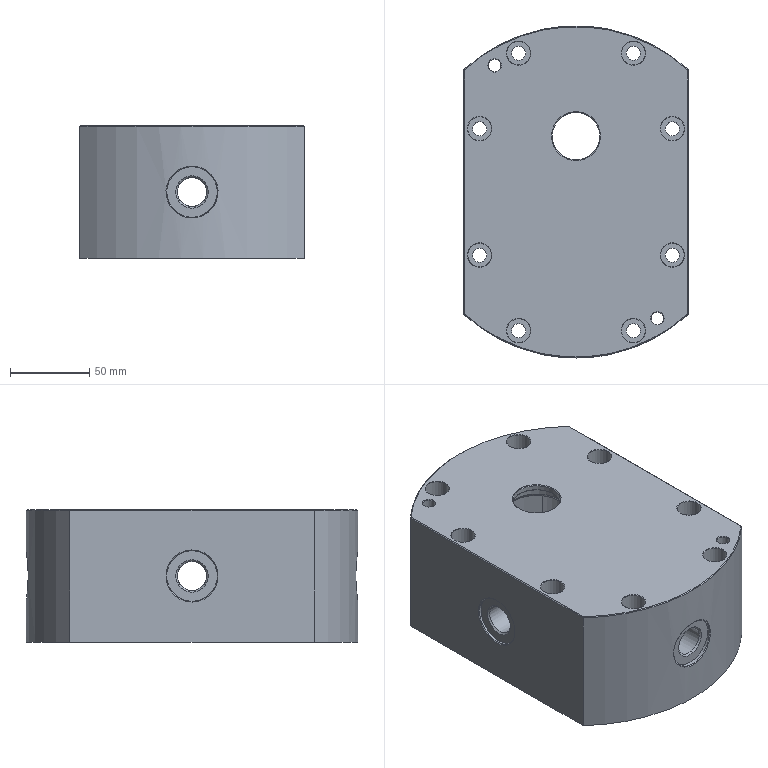NC program | NX | posted with a generic post | part box 142 x 210 x 84 mm
Lines 1512 to 1634 of 1634:
(HOLE_MILLING_COPY_1_COPY_1 , TOOL : D10JING)
N3016 T11 M6
N3018 G54
N3020 G17 G0 G90 X35.25 Y0. B0. C0. S5000 M3
N3022 G43 Z30. H11
N3024 Z-12.
N3026 G94 G1 X32.801 Y-6.451 F1000.
N3028 G3 X35.25 Y-10. R2.619
N3030 X45.25 Y0. R10.
N3032 X35.25 Y-10. R-10.
N3034 X37.699 Y-6.451 R2.619
N3036 G1 X35.25 Y0.
N3038 G0 Z30.
N3040 M5
(PLANAR_MILL_COPY_COPY , TOOL : D6A45)
N3042 T07 M6
N3044 G54
N3046 G17 G0 G90 X92.513 Y-38.084 B0. C0. S7500 M3
N3048 G43 Z30. H7
N3050 Z1.5
N3052 G94 G1 Z-1.5 F1250.
N3054 X93.661 Y-37.121
N3056 G3 X94.019 Y-36.355 R1.
N3058 X87.769 Y-30.105 R6.25
N3060 X94.019 Y-36.355 R-6.25
N3062 X93.661 Y-35.589 R1.
N3064 G1 X92.513 Y-34.625
N3066 Z1.5
N3068 G0 Z30.
N3070 X38.271 Y-65.745
N3072 Z1.5
N3074 G1 Z-1.5
N3076 X39.234 Y-66.893
N3078 G3 X40. Y-67.25 R1.
N3080 X46.25 Y-61. R6.25
N3082 X40. Y-67.25 R-6.25
N3084 X40.766 Y-66.893 R1.
N3086 G1 X41.729 Y-65.745
N3088 Z1.5
N3090 G0 Z30.
N3092 X33.697 Y-12.705
N3094 Z1.5
N3096 G1 Z-1.5
N3098 X34.484 Y-13.643
N3100 G3 X35.25 Y-14. R1.
N3102 X49.25 Y0. R14.
N3104 X35.25 Y-14. R-14.
N3106 X36.016 Y-13.643 R1.
N3108 G1 X36.803 Y-12.705
N3110 Z1.5
N3112 G0 Z30.
N3114 X92.513 Y34.625
N3116 Z1.5
N3118 G1 Z-1.5
N3120 X93.661 Y35.589
N3122 G3 X94.019 Y36.355 R1.
N3124 X87.769 Y42.605 R6.25
N3126 X94.019 Y36.355 R-6.25
N3128 X93.661 Y37.121 R1.
N3130 G1 X92.513 Y38.084
N3132 Z1.5
N3134 G0 Z30.
N3136 X41.729 Y65.745
N3138 Z1.5
N3140 G1 Z-1.5
N3142 X40.766 Y66.893
N3144 G3 X40. Y67.25 R1.
N3146 X33.75 Y61. R6.25
N3148 X40. Y67.25 R-6.25
N3150 X39.234 Y66.893 R1.
N3152 G1 X38.271 Y65.745
N3154 Z1.5
N3156 G0 Z30.
N3158 X-38.271
N3160 Z1.5
N3162 G1 Z-1.5
N3164 X-39.234 Y66.893
N3166 G3 X-40. Y67.25 R1.
N3168 X-46.25 Y61. R6.25
N3170 X-40. Y67.25 R-6.25
N3172 X-40.766 Y66.893 R1.
N3174 G1 X-41.729 Y65.745
N3176 Z1.5
N3178 G0 Z30.
N3180 X-92.513 Y38.084
N3182 Z1.5
N3184 G1 Z-1.5
N3186 X-93.661 Y37.121
N3188 G3 X-94.019 Y36.355 R1.
N3190 X-87.769 Y30.105 R6.25
N3192 X-94.019 Y36.355 R-6.25
N3194 X-93.661 Y35.589 R1.
N3196 G1 X-92.513 Y34.625
N3198 Z1.5
N3200 G0 Z30.
N3202 Y-34.625
N3204 Z1.5
N3206 G1 Z-1.5
N3208 X-93.661 Y-35.589
N3210 G3 X-94.019 Y-36.355 R1.
N3212 X-87.769 Y-42.605 R6.25
N3214 X-94.019 Y-36.355 R-6.25
N3216 X-93.661 Y-37.121 R1.
N3218 G1 X-92.513 Y-38.084
N3220 Z1.5
N3222 G0 Z30.
N3224 X-41.729 Y-65.745
N3226 Z1.5
N3228 G1 Z-1.5
N3230 X-40.766 Y-66.893
N3232 G3 X-40. Y-67.25 R1.
N3234 X-33.75 Y-61. R6.25
N3236 X-40. Y-67.25 R-6.25
N3238 X-39.234 Y-66.893 R1.
N3240 G1 X-38.271 Y-65.745
N3242 Z1.5
N3244 G0 Z30.
N3246 M5
N3248 M2